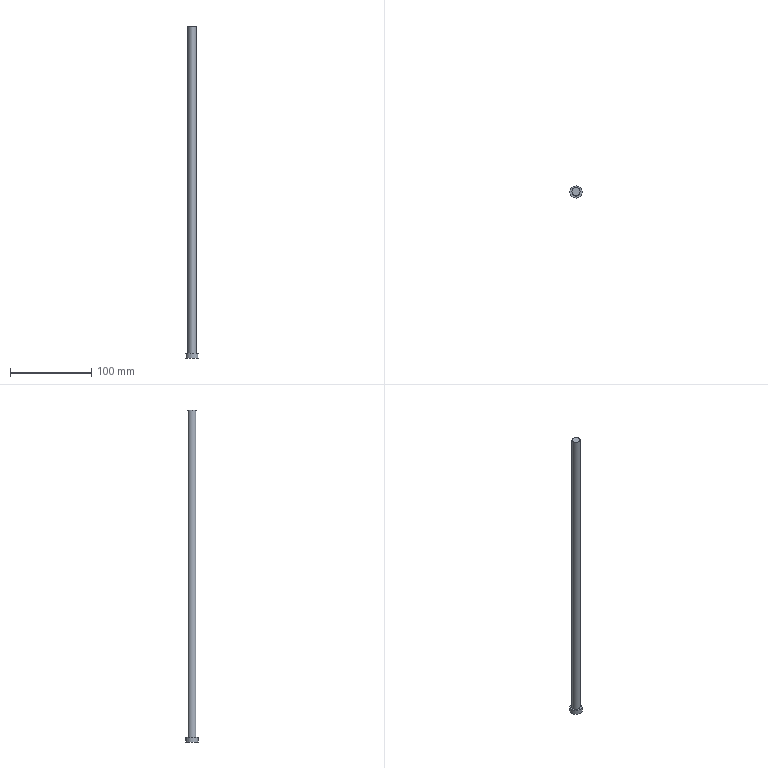Part | STEP file | solid 68 | 1 solid | 5 faces | box 15 x 15 x 408.49 mm | volume 32672 mm3 | plane 3 | cylinder 2 | commonest cylinder face diameters 10 x1 15 x1